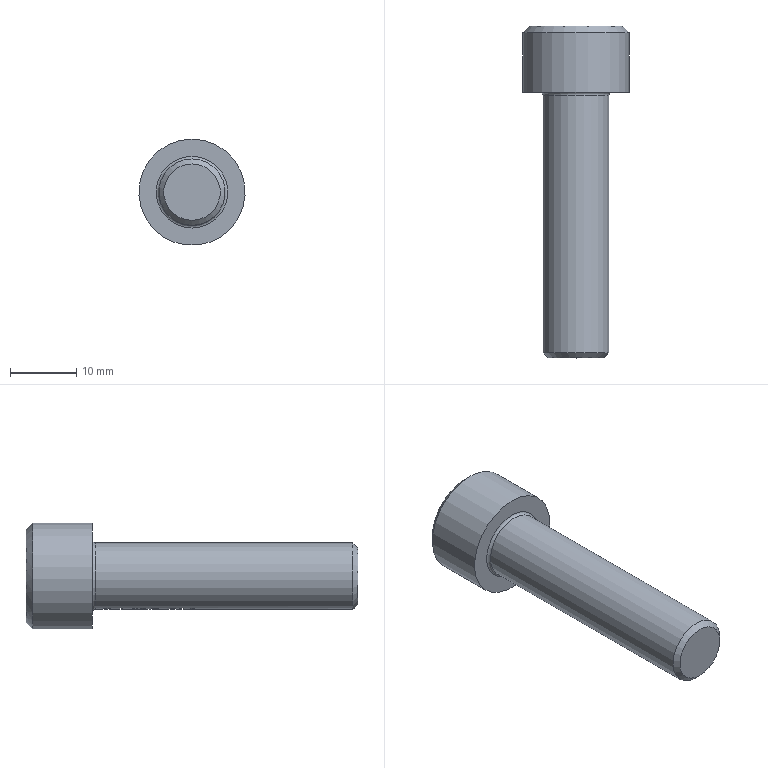Part | STEP file | solid 147 | 1 solid | 108 faces | box 16 x 50 x 16 mm | volume 4838 mm3 | plane 67 | other 24 | cylinder 8 | sphere 6 | cone 2 | torus 1 | commonest cylinder face diameters 10 x7 16 x1